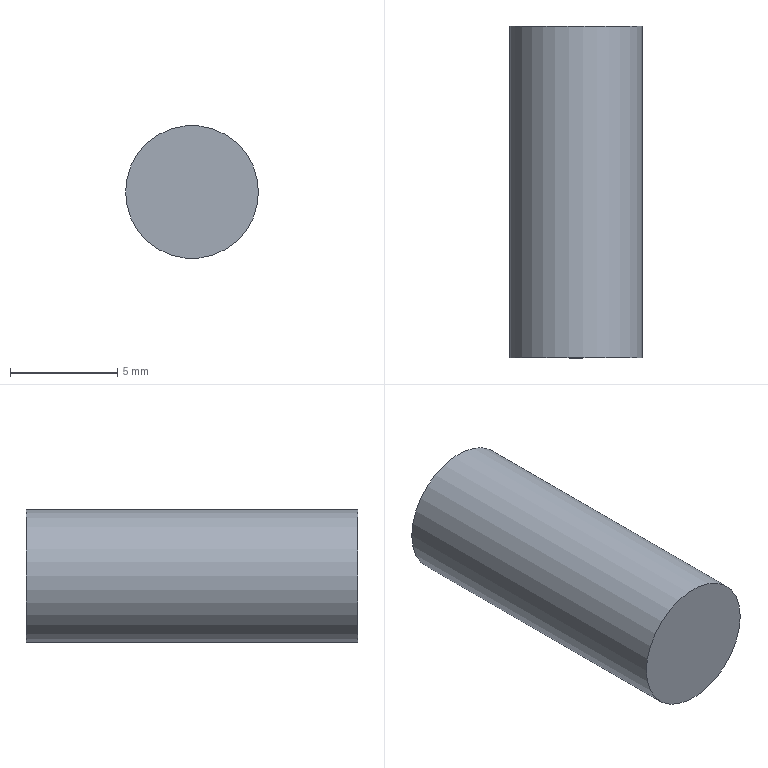Part | STEP file | basic_gh_motor_gh1_07 | 1 solid | 3 faces | box 6.2 x 15.48 x 6.2 mm | volume 467.352 mm3 | plane 2 | cylinder 1 | commonest cylinder face diameters 6.2 x1
STEP:
#1=CARTESIAN_POINT('',(-209.35,124.1,0.));
#2=VERTEX_POINT('',#1);
#3=CARTESIAN_POINT('',(-206.25,124.1,0.));
#4=DIRECTION('',(0.,-1.,0.));
#5=DIRECTION('',(1.,0.,0.));
#6=AXIS2_PLACEMENT_3D('',#3,#4,#5);
#7=CIRCLE('',#6,3.1);
#8=EDGE_CURVE('',#2,#2,#7,.T.);
#9=ORIENTED_EDGE('',*,*,#8,.F.);
#10=CARTESIAN_POINT('',(-209.35,139.58,0.));
#11=VERTEX_POINT('',#10);
#12=CARTESIAN_POINT('',(-209.35,131.84,0.));
#13=DIRECTION('',(0.,1.,0.));
#14=VECTOR('',#13,3.1);
#15=LINE('',#12,#14);
#16=EDGE_CURVE('',#2,#11,#15,.T.);
#17=ORIENTED_EDGE('',*,*,#16,.T.);
#18=CARTESIAN_POINT('',(-206.25,139.58,0.));
#19=DIRECTION('',(0.,1.,0.));
#20=DIRECTION('',(1.,0.,0.));
#21=AXIS2_PLACEMENT_3D('',#18,#19,#20);
#22=CIRCLE('',#21,3.1);
#23=EDGE_CURVE('',#11,#11,#22,.T.);
#24=ORIENTED_EDGE('',*,*,#23,.F.);
#25=ORIENTED_EDGE('',*,*,#16,.F.);
#26=EDGE_LOOP('',(#9,#17,#24,#25));
#27=FACE_OUTER_BOUND('',#26,.T.);
#28=CARTESIAN_POINT('',(-206.25,131.84,0.));
#29=DIRECTION('',(0.,-1.,0.));
#30=DIRECTION('',(1.,0.,0.));
#31=AXIS2_PLACEMENT_3D('',#28,#29,#30);
#32=CYLINDRICAL_SURFACE('',#31,3.1);
#33=ADVANCED_FACE('',(#27),#32,.T.);
#34=ORIENTED_EDGE('',*,*,#23,.T.);
#35=EDGE_LOOP('',(#34));
#36=FACE_OUTER_BOUND('',#35,.T.);
#37=CARTESIAN_POINT('',(-206.25,139.58,0.));
#38=DIRECTION('',(0.,1.,0.));
#39=DIRECTION('',(-1.,0.,0.));
#40=AXIS2_PLACEMENT_3D('',#37,#38,#39);
#41=PLANE('',#40);
#42=ADVANCED_FACE('',(#36),#41,.T.);
#43=ORIENTED_EDGE('',*,*,#8,.T.);
#44=EDGE_LOOP('',(#43));
#45=FACE_OUTER_BOUND('',#44,.T.);
#46=CARTESIAN_POINT('',(-206.25,124.1,0.));
#47=DIRECTION('',(0.,-1.,0.));
#48=DIRECTION('',(1.,0.,0.));
#49=AXIS2_PLACEMENT_3D('',#46,#47,#48);
#50=PLANE('',#49);
#51=ADVANCED_FACE('',(#45),#50,.T.);
#52=CLOSED_SHELL('',(#33,#42,#51));
#53=MANIFOLD_SOLID_BREP('',#52);
#54=(LENGTH_UNIT()NAMED_UNIT(*)SI_UNIT(.MILLI.,.METRE.));
#55=UNCERTAINTY_MEASURE_WITH_UNIT(LENGTH_MEASURE(0.01),#54,'','');
#56=(NAMED_UNIT(*)PLANE_ANGLE_UNIT()SI_UNIT($,.RADIAN.));
#57=(NAMED_UNIT(*)SI_UNIT($,.STERADIAN.)SOLID_ANGLE_UNIT());
#58=(GEOMETRIC_REPRESENTATION_CONTEXT(3)GLOBAL_UNCERTAINTY_ASSIGNED_CONTEXT((#55))GLOBAL_UNIT_ASSIGNED_CONTEXT((#54,#56,#57))REPRESENTATION_CONTEXT('',''));
#59=ADVANCED_BREP_SHAPE_REPRESENTATION('',(#53),#58);